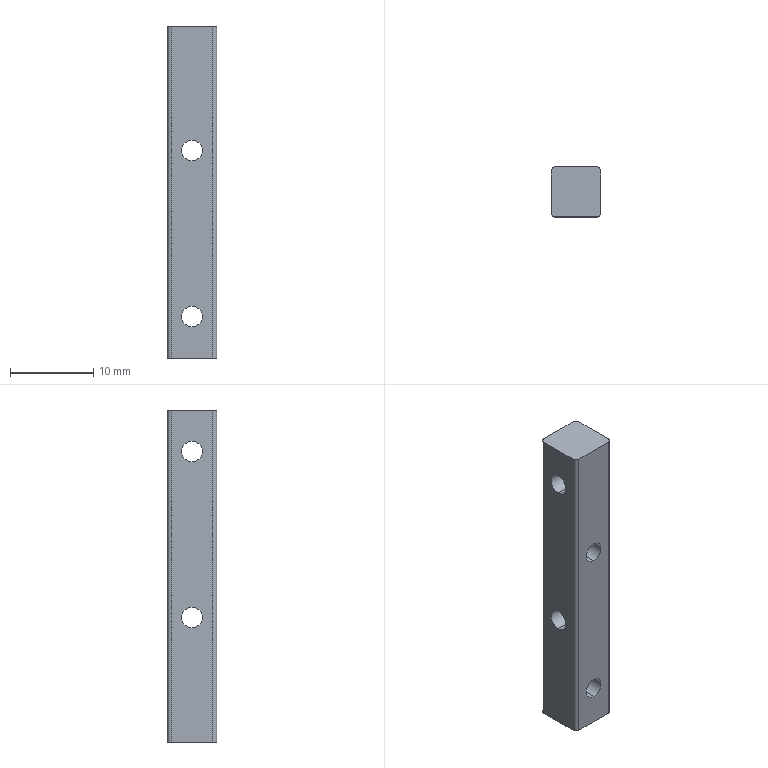Part | SolidWorks | features HoleWzd 2, Extrusion 1, Fillet 1 | 1 solid | 18 faces | box 6 x 6 x 40 mm | volume 1314 mm3 | cylinder 12 | plane 6 | commonest cylinder face diameters 2.5 x8 1 x4
STEP:
#1=CARTESIAN_POINT('',(-3.,0.,16.25));
#2=VERTEX_POINT('',#1);
#3=CARTESIAN_POINT('',(-3.,0.,13.75));
#4=VERTEX_POINT('',#3);
#5=CARTESIAN_POINT('',(-3.,0.,15.));
#6=DIRECTION('',(1.,0.,0.));
#7=DIRECTION('',(0.,0.,-1.));
#8=AXIS2_PLACEMENT_3D('',#5,#6,#7);
#9=CIRCLE('',#8,1.25);
#10=EDGE_CURVE('',#2,#4,#9,.T.);
#11=ORIENTED_EDGE('',*,*,#10,.F.);
#12=CARTESIAN_POINT('',(3.,0.,16.25));
#13=VERTEX_POINT('',#12);
#14=CARTESIAN_POINT('',(3.,0.,16.25));
#15=DIRECTION('',(1.,0.,0.));
#16=VECTOR('',#15,1000.);
#17=LINE('',#14,#16);
#18=EDGE_CURVE('',#2,#13,#17,.T.);
#19=ORIENTED_EDGE('',*,*,#18,.T.);
#20=CARTESIAN_POINT('',(3.,0.,13.75));
#21=VERTEX_POINT('',#20);
#22=CARTESIAN_POINT('',(3.,0.,15.));
#23=DIRECTION('',(1.,0.,0.));
#24=DIRECTION('',(0.,0.,-1.));
#25=AXIS2_PLACEMENT_3D('',#22,#23,#24);
#26=CIRCLE('',#25,1.25);
#27=EDGE_CURVE('',#13,#21,#26,.T.);
#28=ORIENTED_EDGE('',*,*,#27,.T.);
#29=CARTESIAN_POINT('',(3.,0.,13.75));
#30=DIRECTION('',(1.,0.,0.));
#31=VECTOR('',#30,1000.);
#32=LINE('',#29,#31);
#33=EDGE_CURVE('',#4,#21,#32,.T.);
#34=ORIENTED_EDGE('',*,*,#33,.F.);
#35=EDGE_LOOP('',(#11,#19,#28,#34));
#36=FACE_OUTER_BOUND('',#35,.T.);
#37=CARTESIAN_POINT('',(3.,0.,15.));
#38=DIRECTION('',(1.,0.,0.));
#39=DIRECTION('',(0.,0.,-1.));
#40=AXIS2_PLACEMENT_3D('',#37,#38,#39);
#41=CYLINDRICAL_SURFACE('',#40,1.25);
#42=ADVANCED_FACE('',(#36),#41,.F.);
#43=CARTESIAN_POINT('',(-3.,0.,-3.75));
#44=VERTEX_POINT('',#43);
#45=CARTESIAN_POINT('',(-3.,0.,-6.25));
#46=VERTEX_POINT('',#45);
#47=CARTESIAN_POINT('',(-3.,0.,-5.));
#48=DIRECTION('',(1.,0.,0.));
#49=DIRECTION('',(0.,0.,-1.));
#50=AXIS2_PLACEMENT_3D('',#47,#48,#49);
#51=CIRCLE('',#50,1.25);
#52=EDGE_CURVE('',#44,#46,#51,.T.);
#53=ORIENTED_EDGE('',*,*,#52,.F.);
#54=CARTESIAN_POINT('',(3.,0.,-3.75));
#55=VERTEX_POINT('',#54);
#56=CARTESIAN_POINT('',(3.,0.,-3.75));
#57=DIRECTION('',(1.,0.,0.));
#58=VECTOR('',#57,1000.);
#59=LINE('',#56,#58);
#60=EDGE_CURVE('',#44,#55,#59,.T.);
#61=ORIENTED_EDGE('',*,*,#60,.T.);
#62=CARTESIAN_POINT('',(3.,0.,-6.25));
#63=VERTEX_POINT('',#62);
#64=CARTESIAN_POINT('',(3.,0.,-5.));
#65=DIRECTION('',(1.,0.,0.));
#66=DIRECTION('',(0.,0.,-1.));
#67=AXIS2_PLACEMENT_3D('',#64,#65,#66);
#68=CIRCLE('',#67,1.25);
#69=EDGE_CURVE('',#55,#63,#68,.T.);
#70=ORIENTED_EDGE('',*,*,#69,.T.);
#71=CARTESIAN_POINT('',(3.,0.,-6.25));
#72=DIRECTION('',(1.,0.,0.));
#73=VECTOR('',#72,1000.);
#74=LINE('',#71,#73);
#75=EDGE_CURVE('',#46,#63,#74,.T.);
#76=ORIENTED_EDGE('',*,*,#75,.F.);
#77=EDGE_LOOP('',(#53,#61,#70,#76));
#78=FACE_OUTER_BOUND('',#77,.T.);
#79=CARTESIAN_POINT('',(3.,0.,-5.));
#80=DIRECTION('',(1.,0.,0.));
#81=DIRECTION('',(0.,0.,-1.));
#82=AXIS2_PLACEMENT_3D('',#79,#80,#81);
#83=CYLINDRICAL_SURFACE('',#82,1.25);
#84=ADVANCED_FACE('',(#78),#83,.F.);
#85=CARTESIAN_POINT('',(0.,-3.,-16.25));
#86=VERTEX_POINT('',#85);
#87=CARTESIAN_POINT('',(0.,-3.,-13.75));
#88=VERTEX_POINT('',#87);
#89=CARTESIAN_POINT('',(0.,-3.,-15.));
#90=DIRECTION('',(0.,1.,0.));
#91=DIRECTION('',(0.,0.,1.));
#92=AXIS2_PLACEMENT_3D('',#89,#90,#91);
#93=CIRCLE('',#92,1.25);
#94=EDGE_CURVE('',#86,#88,#93,.T.);
#95=ORIENTED_EDGE('',*,*,#94,.F.);
#96=CARTESIAN_POINT('',(0.,3.,-16.25));
#97=VERTEX_POINT('',#96);
#98=CARTESIAN_POINT('',(0.,3.,-16.25));
#99=DIRECTION('',(0.,1.,0.));
#100=VECTOR('',#99,1000.);
#101=LINE('',#98,#100);
#102=EDGE_CURVE('',#86,#97,#101,.T.);
#103=ORIENTED_EDGE('',*,*,#102,.T.);
#104=CARTESIAN_POINT('',(0.,3.,-13.75));
#105=VERTEX_POINT('',#104);
#106=CARTESIAN_POINT('',(0.,3.,-15.));
#107=DIRECTION('',(0.,1.,0.));
#108=DIRECTION('',(0.,0.,1.));
#109=AXIS2_PLACEMENT_3D('',#106,#107,#108);
#110=CIRCLE('',#109,1.25);
#111=EDGE_CURVE('',#97,#105,#110,.T.);
#112=ORIENTED_EDGE('',*,*,#111,.T.);
#113=CARTESIAN_POINT('',(0.,3.,-13.75));
#114=DIRECTION('',(0.,1.,0.));
#115=VECTOR('',#114,1000.);
#116=LINE('',#113,#115);
#117=EDGE_CURVE('',#88,#105,#116,.T.);
#118=ORIENTED_EDGE('',*,*,#117,.F.);
#119=EDGE_LOOP('',(#95,#103,#112,#118));
#120=FACE_OUTER_BOUND('',#119,.T.);
#121=CARTESIAN_POINT('',(0.,3.,-15.));
#122=DIRECTION('',(0.,1.,0.));
#123=DIRECTION('',(0.,0.,1.));
#124=AXIS2_PLACEMENT_3D('',#121,#122,#123);
#125=CYLINDRICAL_SURFACE('',#124,1.25);
#126=ADVANCED_FACE('',(#120),#125,.F.);
#127=CARTESIAN_POINT('',(0.,-3.,3.75));
#128=VERTEX_POINT('',#127);
#129=CARTESIAN_POINT('',(0.,-3.,6.25));
#130=VERTEX_POINT('',#129);
#131=CARTESIAN_POINT('',(0.,-3.,5.));
#132=DIRECTION('',(0.,1.,0.));
#133=DIRECTION('',(0.,0.,1.));
#134=AXIS2_PLACEMENT_3D('',#131,#132,#133);
#135=CIRCLE('',#134,1.25);
#136=EDGE_CURVE('',#128,#130,#135,.T.);
#137=ORIENTED_EDGE('',*,*,#136,.F.);
#138=CARTESIAN_POINT('',(0.,3.,3.75));
#139=VERTEX_POINT('',#138);
#140=CARTESIAN_POINT('',(0.,3.,3.75));
#141=DIRECTION('',(0.,1.,0.));
#142=VECTOR('',#141,1000.);
#143=LINE('',#140,#142);
#144=EDGE_CURVE('',#128,#139,#143,.T.);
#145=ORIENTED_EDGE('',*,*,#144,.T.);
#146=CARTESIAN_POINT('',(0.,3.,6.25));
#147=VERTEX_POINT('',#146);
#148=CARTESIAN_POINT('',(0.,3.,5.));
#149=DIRECTION('',(0.,1.,0.));
#150=DIRECTION('',(0.,0.,1.));
#151=AXIS2_PLACEMENT_3D('',#148,#149,#150);
#152=CIRCLE('',#151,1.25);
#153=EDGE_CURVE('',#139,#147,#152,.T.);
#154=ORIENTED_EDGE('',*,*,#153,.T.);
#155=CARTESIAN_POINT('',(0.,3.,6.25));
#156=DIRECTION('',(0.,1.,0.));
#157=VECTOR('',#156,1000.);
#158=LINE('',#155,#157);
#159=EDGE_CURVE('',#130,#147,#158,.T.);
#160=ORIENTED_EDGE('',*,*,#159,.F.);
#161=EDGE_LOOP('',(#137,#145,#154,#160));
#162=FACE_OUTER_BOUND('',#161,.T.);
#163=CARTESIAN_POINT('',(0.,3.,5.));
#164=DIRECTION('',(0.,1.,0.));
#165=DIRECTION('',(0.,0.,1.));
#166=AXIS2_PLACEMENT_3D('',#163,#164,#165);
#167=CYLINDRICAL_SURFACE('',#166,1.25);
#168=ADVANCED_FACE('',(#162),#167,.F.);
#169=CARTESIAN_POINT('',(0.,3.,5.));
#170=DIRECTION('',(0.,1.,0.));
#171=DIRECTION('',(0.,0.,1.));
#172=AXIS2_PLACEMENT_3D('',#169,#170,#171);
#173=CIRCLE('',#172,1.25);
#174=EDGE_CURVE('',#147,#139,#173,.T.);
#175=ORIENTED_EDGE('',*,*,#174,.F.);
#176=ORIENTED_EDGE('',*,*,#153,.F.);
#177=EDGE_LOOP('',(#175,#176));
#178=FACE_BOUND('',#177,.T.);
#179=CARTESIAN_POINT('',(2.5,3.,-20.));
#180=VERTEX_POINT('',#179);
#181=CARTESIAN_POINT('',(-2.5,3.,-20.));
#182=VERTEX_POINT('',#181);
#183=CARTESIAN_POINT('',(-3.,3.,-20.));
#184=DIRECTION('',(-1.,0.,0.));
#185=VECTOR('',#184,1000.);
#186=LINE('',#183,#185);
#187=EDGE_CURVE('',#180,#182,#186,.T.);
#188=ORIENTED_EDGE('',*,*,#187,.T.);
#189=CARTESIAN_POINT('',(-2.5,3.,20.));
#190=VERTEX_POINT('',#189);
#191=CARTESIAN_POINT('',(-2.5,3.,20.));
#192=DIRECTION('',(0.,0.,1.));
#193=VECTOR('',#192,1000.);
#194=LINE('',#191,#193);
#195=EDGE_CURVE('',#182,#190,#194,.T.);
#196=ORIENTED_EDGE('',*,*,#195,.T.);
#197=CARTESIAN_POINT('',(2.5,3.,20.));
#198=VERTEX_POINT('',#197);
#199=CARTESIAN_POINT('',(-3.,3.,20.));
#200=DIRECTION('',(-1.,0.,0.));
#201=VECTOR('',#200,1000.);
#202=LINE('',#199,#201);
#203=EDGE_CURVE('',#198,#190,#202,.T.);
#204=ORIENTED_EDGE('',*,*,#203,.F.);
#205=CARTESIAN_POINT('',(2.5,3.,20.));
#206=DIRECTION('',(0.,0.,-1.));
#207=VECTOR('',#206,1000.);
#208=LINE('',#205,#207);
#209=EDGE_CURVE('',#198,#180,#208,.T.);
#210=ORIENTED_EDGE('',*,*,#209,.T.);
#211=EDGE_LOOP('',(#188,#196,#204,#210));
#212=FACE_OUTER_BOUND('',#211,.T.);
#213=CARTESIAN_POINT('',(0.,3.,-15.));
#214=DIRECTION('',(0.,1.,0.));
#215=DIRECTION('',(0.,0.,1.));
#216=AXIS2_PLACEMENT_3D('',#213,#214,#215);
#217=CIRCLE('',#216,1.25);
#218=EDGE_CURVE('',#105,#97,#217,.T.);
#219=ORIENTED_EDGE('',*,*,#218,.F.);
#220=ORIENTED_EDGE('',*,*,#111,.F.);
#221=EDGE_LOOP('',(#219,#220));
#222=FACE_BOUND('',#221,.T.);
#223=CARTESIAN_POINT('',(-3.,3.,20.));
#224=DIRECTION('',(0.,-1.,0.));
#225=DIRECTION('',(0.,0.,-1.));
#226=AXIS2_PLACEMENT_3D('',#223,#224,#225);
#227=PLANE('',#226);
#228=ADVANCED_FACE('',(#178,#212,#222),#227,.F.);
#229=CARTESIAN_POINT('',(3.,0.,15.));
#230=DIRECTION('',(1.,0.,0.));
#231=DIRECTION('',(0.,0.,-1.));
#232=AXIS2_PLACEMENT_3D('',#229,#230,#231);
#233=CIRCLE('',#232,1.25);
#234=EDGE_CURVE('',#21,#13,#233,.T.);
#235=ORIENTED_EDGE('',*,*,#234,.F.);
#236=ORIENTED_EDGE('',*,*,#27,.F.);
#237=EDGE_LOOP('',(#235,#236));
#238=FACE_BOUND('',#237,.T.);
#239=CARTESIAN_POINT('',(3.,0.,-5.));
#240=DIRECTION('',(1.,0.,0.));
#241=DIRECTION('',(0.,0.,-1.));
#242=AXIS2_PLACEMENT_3D('',#239,#240,#241);
#243=CIRCLE('',#242,1.25);
#244=EDGE_CURVE('',#63,#55,#243,.T.);
#245=ORIENTED_EDGE('',*,*,#244,.F.);
#246=ORIENTED_EDGE('',*,*,#69,.F.);
#247=EDGE_LOOP('',(#245,#246));
#248=FACE_BOUND('',#247,.T.);
#249=CARTESIAN_POINT('',(3.,-2.5,20.));
#250=VERTEX_POINT('',#249);
#251=CARTESIAN_POINT('',(3.,2.5,20.));
#252=VERTEX_POINT('',#251);
#253=CARTESIAN_POINT('',(3.,-3.,20.));
#254=DIRECTION('',(0.,1.,0.));
#255=VECTOR('',#254,1000.);
#256=LINE('',#253,#255);
#257=EDGE_CURVE('',#250,#252,#256,.T.);
#258=ORIENTED_EDGE('',*,*,#257,.F.);
#259=CARTESIAN_POINT('',(3.,-2.5,-20.));
#260=VERTEX_POINT('',#259);
#261=CARTESIAN_POINT('',(3.,-2.5,20.));
#262=DIRECTION('',(0.,0.,-1.));
#263=VECTOR('',#262,1000.);
#264=LINE('',#261,#263);
#265=EDGE_CURVE('',#250,#260,#264,.T.);
#266=ORIENTED_EDGE('',*,*,#265,.T.);
#267=CARTESIAN_POINT('',(3.,2.5,-20.));
#268=VERTEX_POINT('',#267);
#269=CARTESIAN_POINT('',(3.,-3.,-20.));
#270=DIRECTION('',(0.,1.,0.));
#271=VECTOR('',#270,1000.);
#272=LINE('',#269,#271);
#273=EDGE_CURVE('',#260,#268,#272,.T.);
#274=ORIENTED_EDGE('',*,*,#273,.T.);
#275=CARTESIAN_POINT('',(3.,2.5,20.));
#276=DIRECTION('',(0.,0.,1.));
#277=VECTOR('',#276,1000.);
#278=LINE('',#275,#277);
#279=EDGE_CURVE('',#268,#252,#278,.T.);
#280=ORIENTED_EDGE('',*,*,#279,.T.);
#281=EDGE_LOOP('',(#258,#266,#274,#280));
#282=FACE_OUTER_BOUND('',#281,.T.);
#283=CARTESIAN_POINT('',(3.,-3.,20.));
#284=DIRECTION('',(-1.,0.,0.));
#285=DIRECTION('',(0.,0.,1.));
#286=AXIS2_PLACEMENT_3D('',#283,#284,#285);
#287=PLANE('',#286);
#288=ADVANCED_FACE('',(#238,#248,#282),#287,.F.);
#289=CARTESIAN_POINT('',(-3.,0.,15.));
#290=DIRECTION('',(1.,0.,0.));
#291=DIRECTION('',(0.,0.,-1.));
#292=AXIS2_PLACEMENT_3D('',#289,#290,#291);
#293=CIRCLE('',#292,1.25);
#294=EDGE_CURVE('',#4,#2,#293,.T.);
#295=ORIENTED_EDGE('',*,*,#294,.T.);
#296=ORIENTED_EDGE('',*,*,#10,.T.);
#297=EDGE_LOOP('',(#295,#296));
#298=FACE_BOUND('',#297,.T.);
#299=CARTESIAN_POINT('',(-3.,0.,-5.));
#300=DIRECTION('',(1.,0.,0.));
#301=DIRECTION('',(0.,0.,-1.));
#302=AXIS2_PLACEMENT_3D('',#299,#300,#301);
#303=CIRCLE('',#302,1.25);
#304=EDGE_CURVE('',#46,#44,#303,.T.);
#305=ORIENTED_EDGE('',*,*,#304,.T.);
#306=ORIENTED_EDGE('',*,*,#52,.T.);
#307=EDGE_LOOP('',(#305,#306));
#308=FACE_BOUND('',#307,.T.);
#309=CARTESIAN_POINT('',(-3.,2.5,-20.));
#310=VERTEX_POINT('',#309);
#311=CARTESIAN_POINT('',(-3.,-2.5,-20.));
#312=VERTEX_POINT('',#311);
#313=CARTESIAN_POINT('',(-3.,-3.,-20.));
#314=DIRECTION('',(0.,-1.,0.));
#315=VECTOR('',#314,1000.);
#316=LINE('',#313,#315);
#317=EDGE_CURVE('',#310,#312,#316,.T.);
#318=ORIENTED_EDGE('',*,*,#317,.T.);
#319=CARTESIAN_POINT('',(-3.,-2.5,20.));
#320=VERTEX_POINT('',#319);
#321=CARTESIAN_POINT('',(-3.,-2.5,20.));
#322=DIRECTION('',(0.,0.,1.));
#323=VECTOR('',#322,1000.);
#324=LINE('',#321,#323);
#325=EDGE_CURVE('',#312,#320,#324,.T.);
#326=ORIENTED_EDGE('',*,*,#325,.T.);
#327=CARTESIAN_POINT('',(-3.,2.5,20.));
#328=VERTEX_POINT('',#327);
#329=CARTESIAN_POINT('',(-3.,-3.,20.));
#330=DIRECTION('',(0.,-1.,0.));
#331=VECTOR('',#330,1000.);
#332=LINE('',#329,#331);
#333=EDGE_CURVE('',#328,#320,#332,.T.);
#334=ORIENTED_EDGE('',*,*,#333,.F.);
#335=CARTESIAN_POINT('',(-3.,2.5,20.));
#336=DIRECTION('',(0.,0.,-1.));
#337=VECTOR('',#336,1000.);
#338=LINE('',#335,#337);
#339=EDGE_CURVE('',#328,#310,#338,.T.);
#340=ORIENTED_EDGE('',*,*,#339,.T.);
#341=EDGE_LOOP('',(#318,#326,#334,#340));
#342=FACE_OUTER_BOUND('',#341,.T.);
#343=CARTESIAN_POINT('',(-3.,-3.,20.));
#344=DIRECTION('',(1.,0.,0.));
#345=DIRECTION('',(0.,0.,-1.));
#346=AXIS2_PLACEMENT_3D('',#343,#344,#345);
#347=PLANE('',#346);
#348=ADVANCED_FACE('',(#298,#308,#342),#347,.F.);
#349=CARTESIAN_POINT('',(0.,-3.,-15.));
#350=DIRECTION('',(0.,1.,0.));
#351=DIRECTION('',(0.,0.,1.));
#352=AXIS2_PLACEMENT_3D('',#349,#350,#351);
#353=CIRCLE('',#352,1.25);
#354=EDGE_CURVE('',#88,#86,#353,.T.);
#355=ORIENTED_EDGE('',*,*,#354,.T.);
#356=ORIENTED_EDGE('',*,*,#94,.T.);
#357=EDGE_LOOP('',(#355,#356));
#358=FACE_BOUND('',#357,.T.);
#359=CARTESIAN_POINT('',(0.,-3.,5.));
#360=DIRECTION('',(0.,1.,0.));
#361=DIRECTION('',(0.,0.,1.));
#362=AXIS2_PLACEMENT_3D('',#359,#360,#361);
#363=CIRCLE('',#362,1.25);
#364=EDGE_CURVE('',#130,#128,#363,.T.);
#365=ORIENTED_EDGE('',*,*,#364,.T.);
#366=ORIENTED_EDGE('',*,*,#136,.T.);
#367=EDGE_LOOP('',(#365,#366));
#368=FACE_BOUND('',#367,.T.);
#369=CARTESIAN_POINT('',(-2.5,-3.,-20.));
#370=VERTEX_POINT('',#369);
#371=CARTESIAN_POINT('',(2.5,-3.,-20.));
#372=VERTEX_POINT('',#371);
#373=CARTESIAN_POINT('',(-3.,-3.,-20.));
#374=DIRECTION('',(1.,0.,0.));
#375=VECTOR('',#374,1000.);
#376=LINE('',#373,#375);
#377=EDGE_CURVE('',#370,#372,#376,.T.);
#378=ORIENTED_EDGE('',*,*,#377,.T.);
#379=CARTESIAN_POINT('',(2.5,-3.,20.));
#380=VERTEX_POINT('',#379);
#381=CARTESIAN_POINT('',(2.5,-3.,20.));
#382=DIRECTION('',(0.,0.,1.));
#383=VECTOR('',#382,1000.);
#384=LINE('',#381,#383);
#385=EDGE_CURVE('',#372,#380,#384,.T.);
#386=ORIENTED_EDGE('',*,*,#385,.T.);
#387=CARTESIAN_POINT('',(-2.5,-3.,20.));
#388=VERTEX_POINT('',#387);
#389=CARTESIAN_POINT('',(-3.,-3.,20.));
#390=DIRECTION('',(1.,0.,0.));
#391=VECTOR('',#390,1000.);
#392=LINE('',#389,#391);
#393=EDGE_CURVE('',#388,#380,#392,.T.);
#394=ORIENTED_EDGE('',*,*,#393,.F.);
#395=CARTESIAN_POINT('',(-2.5,-3.,20.));
#396=DIRECTION('',(0.,0.,-1.));
#397=VECTOR('',#396,1000.);
#398=LINE('',#395,#397);
#399=EDGE_CURVE('',#388,#370,#398,.T.);
#400=ORIENTED_EDGE('',*,*,#399,.T.);
#401=EDGE_LOOP('',(#378,#386,#394,#400));
#402=FACE_OUTER_BOUND('',#401,.T.);
#403=CARTESIAN_POINT('',(-3.,-3.,20.));
#404=DIRECTION('',(0.,1.,0.));
#405=DIRECTION('',(0.,0.,1.));
#406=AXIS2_PLACEMENT_3D('',#403,#404,#405);
#407=PLANE('',#406);
#408=ADVANCED_FACE('',(#358,#368,#402),#407,.F.);
#409=ORIENTED_EDGE('',*,*,#393,.T.);
#410=CARTESIAN_POINT('',(2.5,-2.5,20.));
#411=DIRECTION('',(0.,0.,1.));
#412=DIRECTION('',(-1.,0.,0.));
#413=AXIS2_PLACEMENT_3D('',#410,#411,#412);
#414=CIRCLE('',#413,0.5);
#415=EDGE_CURVE('',#380,#250,#414,.T.);
#416=ORIENTED_EDGE('',*,*,#415,.T.);
#417=ORIENTED_EDGE('',*,*,#257,.T.);
#418=CARTESIAN_POINT('',(2.5,2.5,20.));
#419=DIRECTION('',(0.,0.,1.));
#420=DIRECTION('',(-1.,0.,0.));
#421=AXIS2_PLACEMENT_3D('',#418,#419,#420);
#422=CIRCLE('',#421,0.5);
#423=EDGE_CURVE('',#252,#198,#422,.T.);
#424=ORIENTED_EDGE('',*,*,#423,.T.);
#425=ORIENTED_EDGE('',*,*,#203,.T.);
#426=CARTESIAN_POINT('',(-2.5,2.5,20.));
#427=DIRECTION('',(0.,0.,1.));
#428=DIRECTION('',(-1.,0.,0.));
#429=AXIS2_PLACEMENT_3D('',#426,#427,#428);
#430=CIRCLE('',#429,0.5);
#431=EDGE_CURVE('',#190,#328,#430,.T.);
#432=ORIENTED_EDGE('',*,*,#431,.T.);
#433=ORIENTED_EDGE('',*,*,#333,.T.);
#434=CARTESIAN_POINT('',(-2.5,-2.5,20.));
#435=DIRECTION('',(0.,0.,1.));
#436=DIRECTION('',(-1.,0.,0.));
#437=AXIS2_PLACEMENT_3D('',#434,#435,#436);
#438=CIRCLE('',#437,0.5);
#439=EDGE_CURVE('',#320,#388,#438,.T.);
#440=ORIENTED_EDGE('',*,*,#439,.T.);
#441=EDGE_LOOP('',(#409,#416,#417,#424,#425,#432,#433,#440));
#442=FACE_OUTER_BOUND('',#441,.T.);
#443=CARTESIAN_POINT('',(0.,0.,20.));
#444=DIRECTION('',(0.,0.,-1.));
#445=DIRECTION('',(-1.,0.,0.));
#446=AXIS2_PLACEMENT_3D('',#443,#444,#445);
#447=PLANE('',#446);
#448=ADVANCED_FACE('',(#442),#447,.F.);
#449=ORIENTED_EDGE('',*,*,#273,.F.);
#450=CARTESIAN_POINT('',(2.5,-2.5,-20.));
#451=DIRECTION('',(0.,0.,-1.));
#452=DIRECTION('',(-1.,0.,0.));
#453=AXIS2_PLACEMENT_3D('',#450,#451,#452);
#454=CIRCLE('',#453,0.5);
#455=EDGE_CURVE('',#260,#372,#454,.T.);
#456=ORIENTED_EDGE('',*,*,#455,.T.);
#457=ORIENTED_EDGE('',*,*,#377,.F.);
#458=CARTESIAN_POINT('',(-2.5,-2.5,-20.));
#459=DIRECTION('',(0.,0.,-1.));
#460=DIRECTION('',(-1.,0.,0.));
#461=AXIS2_PLACEMENT_3D('',#458,#459,#460);
#462=CIRCLE('',#461,0.5);
#463=EDGE_CURVE('',#370,#312,#462,.T.);
#464=ORIENTED_EDGE('',*,*,#463,.T.);
#465=ORIENTED_EDGE('',*,*,#317,.F.);
#466=CARTESIAN_POINT('',(-2.5,2.5,-20.));
#467=DIRECTION('',(0.,0.,-1.));
#468=DIRECTION('',(-1.,0.,0.));
#469=AXIS2_PLACEMENT_3D('',#466,#467,#468);
#470=CIRCLE('',#469,0.5);
#471=EDGE_CURVE('',#310,#182,#470,.T.);
#472=ORIENTED_EDGE('',*,*,#471,.T.);
#473=ORIENTED_EDGE('',*,*,#187,.F.);
#474=CARTESIAN_POINT('',(2.5,2.5,-20.));
#475=DIRECTION('',(0.,0.,-1.));
#476=DIRECTION('',(-1.,0.,0.));
#477=AXIS2_PLACEMENT_3D('',#474,#475,#476);
#478=CIRCLE('',#477,0.5);
#479=EDGE_CURVE('',#180,#268,#478,.T.);
#480=ORIENTED_EDGE('',*,*,#479,.T.);
#481=EDGE_LOOP('',(#449,#456,#457,#464,#465,#472,#473,#480));
#482=FACE_OUTER_BOUND('',#481,.T.);
#483=CARTESIAN_POINT('',(0.,0.,-20.));
#484=DIRECTION('',(0.,0.,-1.));
#485=DIRECTION('',(-1.,0.,0.));
#486=AXIS2_PLACEMENT_3D('',#483,#484,#485);
#487=PLANE('',#486);
#488=ADVANCED_FACE('',(#482),#487,.T.);
#489=ORIENTED_EDGE('',*,*,#144,.F.);
#490=ORIENTED_EDGE('',*,*,#364,.F.);
#491=ORIENTED_EDGE('',*,*,#159,.T.);
#492=ORIENTED_EDGE('',*,*,#174,.T.);
#493=EDGE_LOOP('',(#489,#490,#491,#492));
#494=FACE_OUTER_BOUND('',#493,.T.);
#495=CARTESIAN_POINT('',(0.,3.,5.));
#496=DIRECTION('',(0.,1.,0.));
#497=DIRECTION('',(0.,0.,1.));
#498=AXIS2_PLACEMENT_3D('',#495,#496,#497);
#499=CYLINDRICAL_SURFACE('',#498,1.25);
#500=ADVANCED_FACE('',(#494),#499,.F.);
#501=ORIENTED_EDGE('',*,*,#102,.F.);
#502=ORIENTED_EDGE('',*,*,#354,.F.);
#503=ORIENTED_EDGE('',*,*,#117,.T.);
#504=ORIENTED_EDGE('',*,*,#218,.T.);
#505=EDGE_LOOP('',(#501,#502,#503,#504));
#506=FACE_OUTER_BOUND('',#505,.T.);
#507=CARTESIAN_POINT('',(0.,3.,-15.));
#508=DIRECTION('',(0.,1.,0.));
#509=DIRECTION('',(0.,0.,1.));
#510=AXIS2_PLACEMENT_3D('',#507,#508,#509);
#511=CYLINDRICAL_SURFACE('',#510,1.25);
#512=ADVANCED_FACE('',(#506),#511,.F.);
#513=ORIENTED_EDGE('',*,*,#60,.F.);
#514=ORIENTED_EDGE('',*,*,#304,.F.);
#515=ORIENTED_EDGE('',*,*,#75,.T.);
#516=ORIENTED_EDGE('',*,*,#244,.T.);
#517=EDGE_LOOP('',(#513,#514,#515,#516));
#518=FACE_OUTER_BOUND('',#517,.T.);
#519=CARTESIAN_POINT('',(3.,0.,-5.));
#520=DIRECTION('',(1.,0.,0.));
#521=DIRECTION('',(0.,0.,-1.));
#522=AXIS2_PLACEMENT_3D('',#519,#520,#521);
#523=CYLINDRICAL_SURFACE('',#522,1.25);
#524=ADVANCED_FACE('',(#518),#523,.F.);
#525=ORIENTED_EDGE('',*,*,#18,.F.);
#526=ORIENTED_EDGE('',*,*,#294,.F.);
#527=ORIENTED_EDGE('',*,*,#33,.T.);
#528=ORIENTED_EDGE('',*,*,#234,.T.);
#529=EDGE_LOOP('',(#525,#526,#527,#528));
#530=FACE_OUTER_BOUND('',#529,.T.);
#531=CARTESIAN_POINT('',(3.,0.,15.));
#532=DIRECTION('',(1.,0.,0.));
#533=DIRECTION('',(0.,0.,-1.));
#534=AXIS2_PLACEMENT_3D('',#531,#532,#533);
#535=CYLINDRICAL_SURFACE('',#534,1.25);
#536=ADVANCED_FACE('',(#530),#535,.F.);
#537=ORIENTED_EDGE('',*,*,#415,.F.);
#538=ORIENTED_EDGE('',*,*,#385,.F.);
#539=ORIENTED_EDGE('',*,*,#455,.F.);
#540=ORIENTED_EDGE('',*,*,#265,.F.);
#541=EDGE_LOOP('',(#537,#538,#539,#540));
#542=FACE_OUTER_BOUND('',#541,.T.);
#543=CARTESIAN_POINT('',(2.5,-2.5,20.));
#544=DIRECTION('',(0.,0.,-1.));
#545=DIRECTION('',(-1.,0.,0.));
#546=AXIS2_PLACEMENT_3D('',#543,#544,#545);
#547=CYLINDRICAL_SURFACE('',#546,0.5);
#548=ADVANCED_FACE('',(#542),#547,.T.);
#549=ORIENTED_EDGE('',*,*,#439,.F.);
#550=ORIENTED_EDGE('',*,*,#325,.F.);
#551=ORIENTED_EDGE('',*,*,#463,.F.);
#552=ORIENTED_EDGE('',*,*,#399,.F.);
#553=EDGE_LOOP('',(#549,#550,#551,#552));
#554=FACE_OUTER_BOUND('',#553,.T.);
#555=CARTESIAN_POINT('',(-2.5,-2.5,20.));
#556=DIRECTION('',(0.,0.,-1.));
#557=DIRECTION('',(-1.,0.,0.));
#558=AXIS2_PLACEMENT_3D('',#555,#556,#557);
#559=CYLINDRICAL_SURFACE('',#558,0.5);
#560=ADVANCED_FACE('',(#554),#559,.T.);
#561=ORIENTED_EDGE('',*,*,#431,.F.);
#562=ORIENTED_EDGE('',*,*,#195,.F.);
#563=ORIENTED_EDGE('',*,*,#471,.F.);
#564=ORIENTED_EDGE('',*,*,#339,.F.);
#565=EDGE_LOOP('',(#561,#562,#563,#564));
#566=FACE_OUTER_BOUND('',#565,.T.);
#567=CARTESIAN_POINT('',(-2.5,2.5,20.));
#568=DIRECTION('',(0.,0.,-1.));
#569=DIRECTION('',(-1.,0.,0.));
#570=AXIS2_PLACEMENT_3D('',#567,#568,#569);
#571=CYLINDRICAL_SURFACE('',#570,0.5);
#572=ADVANCED_FACE('',(#566),#571,.T.);
#573=ORIENTED_EDGE('',*,*,#423,.F.);
#574=ORIENTED_EDGE('',*,*,#279,.F.);
#575=ORIENTED_EDGE('',*,*,#479,.F.);
#576=ORIENTED_EDGE('',*,*,#209,.F.);
#577=EDGE_LOOP('',(#573,#574,#575,#576));
#578=FACE_OUTER_BOUND('',#577,.T.);
#579=CARTESIAN_POINT('',(2.5,2.5,20.));
#580=DIRECTION('',(0.,0.,-1.));
#581=DIRECTION('',(-1.,0.,0.));
#582=AXIS2_PLACEMENT_3D('',#579,#580,#581);
#583=CYLINDRICAL_SURFACE('',#582,0.5);
#584=ADVANCED_FACE('',(#578),#583,.T.);
#585=CLOSED_SHELL('',(#42,#84,#126,#168,#228,#288,#348,#408,#448,#488,#500,#512,#524,#536,#548,#560,#572,#584));
#586=MANIFOLD_SOLID_BREP('',#585);
#587=CARTESIAN_POINT('',(0.,0.,0.));
#588=DIRECTION('',(0.,0.,1.));
#589=DIRECTION('',(1.,0.,0.));
#590=AXIS2_PLACEMENT_3D('',#587,#588,#589);
#591=(LENGTH_UNIT()NAMED_UNIT(*)SI_UNIT(.MILLI.,.METRE.));
#592=UNCERTAINTY_MEASURE_WITH_UNIT(LENGTH_MEASURE(0.00001),#591,'','');
#593=(NAMED_UNIT(*)PLANE_ANGLE_UNIT()SI_UNIT($,.RADIAN.));
#594=(NAMED_UNIT(*)SI_UNIT($,.STERADIAN.)SOLID_ANGLE_UNIT());
#595=(GEOMETRIC_REPRESENTATION_CONTEXT(3)GLOBAL_UNCERTAINTY_ASSIGNED_CONTEXT((#592))GLOBAL_UNIT_ASSIGNED_CONTEXT((#591,#593,#594))REPRESENTATION_CONTEXT('',''));
#596=ADVANCED_BREP_SHAPE_REPRESENTATION('',(#586,#590),#595);